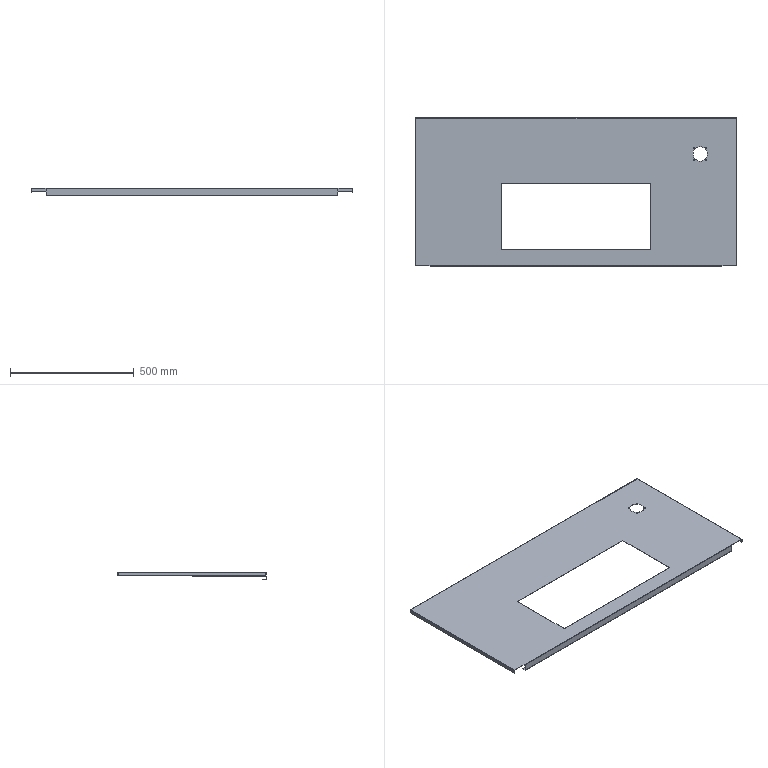Part | SolidWorks | features EdgeFlange 3, ICE 2, FlatPattern 1, SMBaseFlange 1, SheetMetal 1 | 1 solid | 52 faces | box 1298 x 600 x 30 mm | volume 836579 mm3 | plane 28 | cylinder 20 | spline 4 | commonest cylinder face diameters 5 x8 0.9 x5 3.3 x5 58 x2